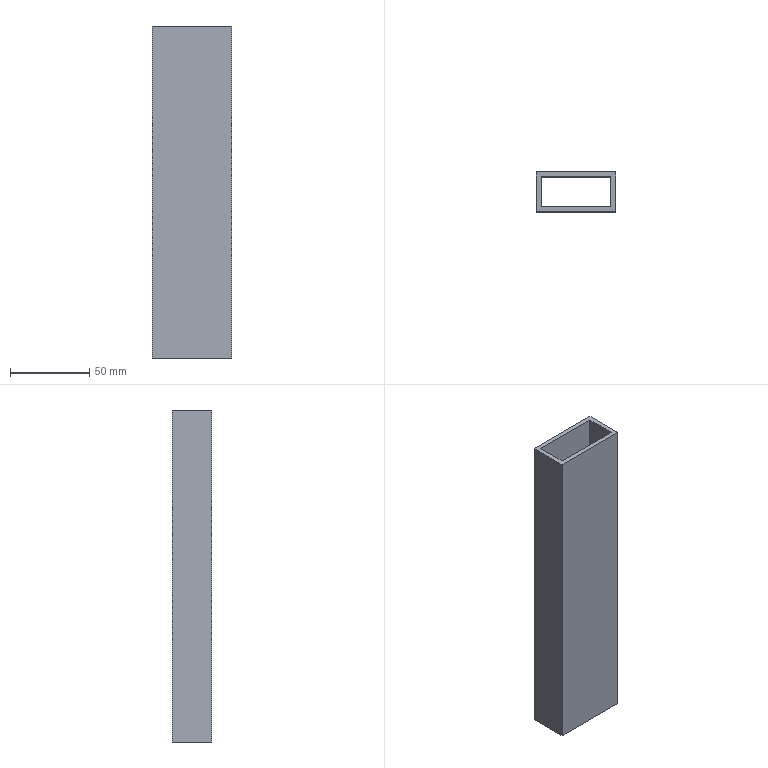Part | STEP file | ASND-0110-E63-HLTP01标准Lower机架-11 | 1 solid | 10 faces | box 50 x 25 x 210 mm | volume 86940 mm3 | plane 10
STEP:
#1=CARTESIAN_POINT('',(0.,0.,0.));
#2=DIRECTION('',(0.,0.,1.));
#3=DIRECTION('',(1.,0.,0.));
#4=AXIS2_PLACEMENT_3D('',#1,#2,#3);
#5=CARTESIAN_POINT('',(-145.,12.5,-210.));
#6=VERTEX_POINT('',#5);
#7=CARTESIAN_POINT('',(-95.,12.5,-210.));
#8=VERTEX_POINT('',#7);
#9=CARTESIAN_POINT('',(-145.,12.5,-210.));
#10=DIRECTION('',(1.,0.,0.));
#11=VECTOR('',#10,1.);
#12=LINE('',#9,#11);
#13=CARTESIAN_POINT('',(-95.,12.5,-265.902));
#14=DIRECTION('',(0.,1.,0.));
#15=DIRECTION('',(0.7071,0.,0.7071));
#16=AXIS2_PLACEMENT_3D('',#13,#14,#15);
#17=PLANE('',#16);
#18=CARTESIAN_POINT('',(4.173,-74.884));
#19=DIRECTION('',(0.7071,0.7071));
#20=VECTOR('',#19,1.);
#21=LINE('',#18,#20);
#22=(GEOMETRIC_REPRESENTATION_CONTEXT(2)PARAMETRIC_REPRESENTATION_CONTEXT()REPRESENTATION_CONTEXT('',''));
#23=DEFINITIONAL_REPRESENTATION('',(#21),#22);
#24=PCURVE('',#17,#23);
#25=CARTESIAN_POINT('',(-200.902,-12.5,-210.));
#26=DIRECTION('',(0.,0.,1.));
#27=DIRECTION('',(0.7071,0.7071,0.));
#28=AXIS2_PLACEMENT_3D('',#25,#26,#27);
#29=PLANE('',#28);
#30=CARTESIAN_POINT('',(57.206,-21.851));
#31=DIRECTION('',(0.7071,-0.7071));
#32=VECTOR('',#31,1.);
#33=LINE('',#30,#32);
#34=(GEOMETRIC_REPRESENTATION_CONTEXT(2)PARAMETRIC_REPRESENTATION_CONTEXT()REPRESENTATION_CONTEXT('',''));
#35=DEFINITIONAL_REPRESENTATION('',(#33),#34);
#36=PCURVE('',#29,#35);
#37=SURFACE_CURVE('',#12,(#24,#36),.PCURVE_S1.);
#38=EDGE_CURVE('',#6,#8,#37,.T.);
#39=ORIENTED_EDGE('',*,*,#38,.F.);
#40=CARTESIAN_POINT('',(-145.,12.5,0.));
#41=VERTEX_POINT('',#40);
#42=CARTESIAN_POINT('',(-145.,12.5,-210.));
#43=DIRECTION('',(0.,0.,1.));
#44=VECTOR('',#43,1.);
#45=LINE('',#42,#44);
#46=CARTESIAN_POINT('',(4.173,-74.884));
#47=DIRECTION('',(0.7071,-0.7071));
#48=VECTOR('',#47,1.);
#49=LINE('',#46,#48);
#50=(GEOMETRIC_REPRESENTATION_CONTEXT(2)PARAMETRIC_REPRESENTATION_CONTEXT()REPRESENTATION_CONTEXT('',''));
#51=DEFINITIONAL_REPRESENTATION('',(#49),#50);
#52=PCURVE('',#17,#51);
#53=CARTESIAN_POINT('',(-145.,12.5,-265.902));
#54=DIRECTION('',(-1.,0.,0.));
#55=DIRECTION('',(0.,0.7071,0.7071));
#56=AXIS2_PLACEMENT_3D('',#53,#54,#55);
#57=PLANE('',#56);
#58=CARTESIAN_POINT('',(39.528,-39.528));
#59=DIRECTION('',(0.7071,-0.7071));
#60=VECTOR('',#59,1.);
#61=LINE('',#58,#60);
#62=(GEOMETRIC_REPRESENTATION_CONTEXT(2)PARAMETRIC_REPRESENTATION_CONTEXT()REPRESENTATION_CONTEXT('',''));
#63=DEFINITIONAL_REPRESENTATION('',(#61),#62);
#64=PCURVE('',#57,#63);
#65=SURFACE_CURVE('',#45,(#52,#64),.PCURVE_S1.);
#66=EDGE_CURVE('',#6,#41,#65,.T.);
#67=ORIENTED_EDGE('',*,*,#66,.T.);
#68=CARTESIAN_POINT('',(-95.,12.5,0.));
#69=VERTEX_POINT('',#68);
#70=CARTESIAN_POINT('',(-95.,12.5,0.));
#71=DIRECTION('',(-1.,0.,0.));
#72=VECTOR('',#71,1.);
#73=LINE('',#70,#72);
#74=CARTESIAN_POINT('',(188.021,-188.021));
#75=DIRECTION('',(-0.7071,-0.7071));
#76=VECTOR('',#75,1.);
#77=LINE('',#74,#76);
#78=(GEOMETRIC_REPRESENTATION_CONTEXT(2)PARAMETRIC_REPRESENTATION_CONTEXT()REPRESENTATION_CONTEXT('',''));
#79=DEFINITIONAL_REPRESENTATION('',(#77),#78);
#80=PCURVE('',#17,#79);
#81=CARTESIAN_POINT('',(0.,0.,0.));
#82=DIRECTION('',(0.,0.,-1.));
#83=DIRECTION('',(0.7071,0.7071,0.));
#84=AXIS2_PLACEMENT_3D('',#81,#82,#83);
#85=PLANE('',#84);
#86=CARTESIAN_POINT('',(-58.336,-76.014));
#87=DIRECTION('',(-0.7071,-0.7071));
#88=VECTOR('',#87,1.);
#89=LINE('',#86,#88);
#90=(GEOMETRIC_REPRESENTATION_CONTEXT(2)PARAMETRIC_REPRESENTATION_CONTEXT()REPRESENTATION_CONTEXT('',''));
#91=DEFINITIONAL_REPRESENTATION('',(#89),#90);
#92=PCURVE('',#85,#91);
#93=SURFACE_CURVE('',#73,(#80,#92),.PCURVE_S1.);
#94=EDGE_CURVE('',#69,#41,#93,.T.);
#95=ORIENTED_EDGE('',*,*,#94,.F.);
#96=CARTESIAN_POINT('',(-95.,12.5,-210.));
#97=DIRECTION('',(0.,0.,1.));
#98=VECTOR('',#97,1.);
#99=LINE('',#96,#98);
#100=CARTESIAN_POINT('',(39.528,-39.528));
#101=DIRECTION('',(0.7071,-0.7071));
#102=VECTOR('',#101,1.);
#103=LINE('',#100,#102);
#104=(GEOMETRIC_REPRESENTATION_CONTEXT(2)PARAMETRIC_REPRESENTATION_CONTEXT()REPRESENTATION_CONTEXT('',''));
#105=DEFINITIONAL_REPRESENTATION('',(#103),#104);
#106=PCURVE('',#17,#105);
#107=CARTESIAN_POINT('',(-95.,12.5,-265.902));
#108=DIRECTION('',(1.,0.,0.));
#109=DIRECTION('',(0.,0.7071,0.7071));
#110=AXIS2_PLACEMENT_3D('',#107,#108,#109);
#111=PLANE('',#110);
#112=CARTESIAN_POINT('',(39.528,39.528));
#113=DIRECTION('',(0.7071,0.7071));
#114=VECTOR('',#113,1.);
#115=LINE('',#112,#114);
#116=(GEOMETRIC_REPRESENTATION_CONTEXT(2)PARAMETRIC_REPRESENTATION_CONTEXT()REPRESENTATION_CONTEXT('',''));
#117=DEFINITIONAL_REPRESENTATION('',(#115),#116);
#118=PCURVE('',#111,#117);
#119=SURFACE_CURVE('',#99,(#106,#118),.PCURVE_S1.);
#120=EDGE_CURVE('',#8,#69,#119,.T.);
#121=ORIENTED_EDGE('',*,*,#120,.F.);
#122=EDGE_LOOP('',(#39,#67,#95,#121));
#123=FACE_BOUND('',#122,.T.);
#124=ADVANCED_FACE('',(#123),#17,.T.);
#125=CARTESIAN_POINT('',(-145.,-12.5,-210.));
#126=VERTEX_POINT('',#125);
#127=CARTESIAN_POINT('',(-145.,-12.5,-210.));
#128=DIRECTION('',(0.,1.,0.));
#129=VECTOR('',#128,1.);
#130=LINE('',#127,#129);
#131=CARTESIAN_POINT('',(21.851,-57.206));
#132=DIRECTION('',(0.7071,0.7071));
#133=VECTOR('',#132,1.);
#134=LINE('',#131,#133);
#135=(GEOMETRIC_REPRESENTATION_CONTEXT(2)PARAMETRIC_REPRESENTATION_CONTEXT()REPRESENTATION_CONTEXT('',''));
#136=DEFINITIONAL_REPRESENTATION('',(#134),#135);
#137=PCURVE('',#57,#136);
#138=CARTESIAN_POINT('',(39.528,-39.528));
#139=DIRECTION('',(0.7071,0.7071));
#140=VECTOR('',#139,1.);
#141=LINE('',#138,#140);
#142=(GEOMETRIC_REPRESENTATION_CONTEXT(2)PARAMETRIC_REPRESENTATION_CONTEXT()REPRESENTATION_CONTEXT('',''));
#143=DEFINITIONAL_REPRESENTATION('',(#141),#142);
#144=PCURVE('',#29,#143);
#145=SURFACE_CURVE('',#130,(#137,#144),.PCURVE_S1.);
#146=EDGE_CURVE('',#126,#6,#145,.T.);
#147=ORIENTED_EDGE('',*,*,#146,.F.);
#148=CARTESIAN_POINT('',(-145.,-12.5,0.));
#149=VERTEX_POINT('',#148);
#150=CARTESIAN_POINT('',(-145.,-12.5,-210.));
#151=DIRECTION('',(0.,0.,1.));
#152=VECTOR('',#151,1.);
#153=LINE('',#150,#152);
#154=CARTESIAN_POINT('',(21.851,-57.206));
#155=DIRECTION('',(0.7071,-0.7071));
#156=VECTOR('',#155,1.);
#157=LINE('',#154,#156);
#158=(GEOMETRIC_REPRESENTATION_CONTEXT(2)PARAMETRIC_REPRESENTATION_CONTEXT()REPRESENTATION_CONTEXT('',''));
#159=DEFINITIONAL_REPRESENTATION('',(#157),#158);
#160=PCURVE('',#57,#159);
#161=CARTESIAN_POINT('',(-95.,-12.5,-265.902));
#162=DIRECTION('',(0.,-1.,0.));
#163=DIRECTION('',(0.7071,0.,0.7071));
#164=AXIS2_PLACEMENT_3D('',#161,#162,#163);
#165=PLANE('',#164);
#166=CARTESIAN_POINT('',(4.173,74.884));
#167=DIRECTION('',(0.7071,0.7071));
#168=VECTOR('',#167,1.);
#169=LINE('',#166,#168);
#170=(GEOMETRIC_REPRESENTATION_CONTEXT(2)PARAMETRIC_REPRESENTATION_CONTEXT()REPRESENTATION_CONTEXT('',''));
#171=DEFINITIONAL_REPRESENTATION('',(#169),#170);
#172=PCURVE('',#165,#171);
#173=SURFACE_CURVE('',#153,(#160,#172),.PCURVE_S1.);
#174=EDGE_CURVE('',#126,#149,#173,.T.);
#175=ORIENTED_EDGE('',*,*,#174,.T.);
#176=CARTESIAN_POINT('',(-145.,12.5,0.));
#177=DIRECTION('',(0.,-1.,0.));
#178=VECTOR('',#177,1.);
#179=LINE('',#176,#178);
#180=CARTESIAN_POINT('',(188.021,-188.021));
#181=DIRECTION('',(-0.7071,-0.7071));
#182=VECTOR('',#181,1.);
#183=LINE('',#180,#182);
#184=(GEOMETRIC_REPRESENTATION_CONTEXT(2)PARAMETRIC_REPRESENTATION_CONTEXT()REPRESENTATION_CONTEXT('',''));
#185=DEFINITIONAL_REPRESENTATION('',(#183),#184);
#186=PCURVE('',#57,#185);
#187=CARTESIAN_POINT('',(-93.692,-111.369));
#188=DIRECTION('',(-0.7071,0.7071));
#189=VECTOR('',#188,1.);
#190=LINE('',#187,#189);
#191=(GEOMETRIC_REPRESENTATION_CONTEXT(2)PARAMETRIC_REPRESENTATION_CONTEXT()REPRESENTATION_CONTEXT('',''));
#192=DEFINITIONAL_REPRESENTATION('',(#190),#191);
#193=PCURVE('',#85,#192);
#194=SURFACE_CURVE('',#179,(#186,#193),.PCURVE_S1.);
#195=EDGE_CURVE('',#41,#149,#194,.T.);
#196=ORIENTED_EDGE('',*,*,#195,.F.);
#197=ORIENTED_EDGE('',*,*,#66,.F.);
#198=EDGE_LOOP('',(#147,#175,#196,#197));
#199=FACE_BOUND('',#198,.T.);
#200=ADVANCED_FACE('',(#199),#57,.T.);
#201=CARTESIAN_POINT('',(-95.,-12.5,-210.));
#202=VERTEX_POINT('',#201);
#203=CARTESIAN_POINT('',(-95.,-12.5,-210.));
#204=DIRECTION('',(-1.,0.,0.));
#205=VECTOR('',#204,1.);
#206=LINE('',#203,#205);
#207=CARTESIAN_POINT('',(39.528,39.528));
#208=DIRECTION('',(-0.7071,0.7071));
#209=VECTOR('',#208,1.);
#210=LINE('',#207,#209);
#211=(GEOMETRIC_REPRESENTATION_CONTEXT(2)PARAMETRIC_REPRESENTATION_CONTEXT()REPRESENTATION_CONTEXT('',''));
#212=DEFINITIONAL_REPRESENTATION('',(#210),#211);
#213=PCURVE('',#165,#212);
#214=CARTESIAN_POINT('',(74.884,-74.884));
#215=DIRECTION('',(-0.7071,0.7071));
#216=VECTOR('',#215,1.);
#217=LINE('',#214,#216);
#218=(GEOMETRIC_REPRESENTATION_CONTEXT(2)PARAMETRIC_REPRESENTATION_CONTEXT()REPRESENTATION_CONTEXT('',''));
#219=DEFINITIONAL_REPRESENTATION('',(#217),#218);
#220=PCURVE('',#29,#219);
#221=SURFACE_CURVE('',#206,(#213,#220),.PCURVE_S1.);
#222=EDGE_CURVE('',#202,#126,#221,.T.);
#223=ORIENTED_EDGE('',*,*,#222,.F.);
#224=CARTESIAN_POINT('',(-95.,-12.5,0.));
#225=VERTEX_POINT('',#224);
#226=CARTESIAN_POINT('',(-95.,-12.5,-210.));
#227=DIRECTION('',(0.,0.,1.));
#228=VECTOR('',#227,1.);
#229=LINE('',#226,#228);
#230=CARTESIAN_POINT('',(39.528,39.528));
#231=DIRECTION('',(0.7071,0.7071));
#232=VECTOR('',#231,1.);
#233=LINE('',#230,#232);
#234=(GEOMETRIC_REPRESENTATION_CONTEXT(2)PARAMETRIC_REPRESENTATION_CONTEXT()REPRESENTATION_CONTEXT('',''));
#235=DEFINITIONAL_REPRESENTATION('',(#233),#234);
#236=PCURVE('',#165,#235);
#237=CARTESIAN_POINT('',(21.851,57.206));
#238=DIRECTION('',(0.7071,0.7071));
#239=VECTOR('',#238,1.);
#240=LINE('',#237,#239);
#241=(GEOMETRIC_REPRESENTATION_CONTEXT(2)PARAMETRIC_REPRESENTATION_CONTEXT()REPRESENTATION_CONTEXT('',''));
#242=DEFINITIONAL_REPRESENTATION('',(#240),#241);
#243=PCURVE('',#111,#242);
#244=SURFACE_CURVE('',#229,(#236,#243),.PCURVE_S1.);
#245=EDGE_CURVE('',#202,#225,#244,.T.);
#246=ORIENTED_EDGE('',*,*,#245,.T.);
#247=CARTESIAN_POINT('',(-145.,-12.5,0.));
#248=DIRECTION('',(1.,0.,0.));
#249=VECTOR('',#248,1.);
#250=LINE('',#247,#249);
#251=CARTESIAN_POINT('',(152.666,223.376));
#252=DIRECTION('',(0.7071,-0.7071));
#253=VECTOR('',#252,1.);
#254=LINE('',#251,#253);
#255=(GEOMETRIC_REPRESENTATION_CONTEXT(2)PARAMETRIC_REPRESENTATION_CONTEXT()REPRESENTATION_CONTEXT('',''));
#256=DEFINITIONAL_REPRESENTATION('',(#254),#255);
#257=PCURVE('',#165,#256);
#258=CARTESIAN_POINT('',(-111.369,-93.692));
#259=DIRECTION('',(0.7071,0.7071));
#260=VECTOR('',#259,1.);
#261=LINE('',#258,#260);
#262=(GEOMETRIC_REPRESENTATION_CONTEXT(2)PARAMETRIC_REPRESENTATION_CONTEXT()REPRESENTATION_CONTEXT('',''));
#263=DEFINITIONAL_REPRESENTATION('',(#261),#262);
#264=PCURVE('',#85,#263);
#265=SURFACE_CURVE('',#250,(#257,#264),.PCURVE_S1.);
#266=EDGE_CURVE('',#149,#225,#265,.T.);
#267=ORIENTED_EDGE('',*,*,#266,.F.);
#268=ORIENTED_EDGE('',*,*,#174,.F.);
#269=EDGE_LOOP('',(#223,#246,#267,#268));
#270=FACE_BOUND('',#269,.T.);
#271=ADVANCED_FACE('',(#270),#165,.T.);
#272=CARTESIAN_POINT('',(-95.,12.5,-210.));
#273=DIRECTION('',(0.,-1.,0.));
#274=VECTOR('',#273,1.);
#275=LINE('',#272,#274);
#276=CARTESIAN_POINT('',(39.528,39.528));
#277=DIRECTION('',(-0.7071,0.7071));
#278=VECTOR('',#277,1.);
#279=LINE('',#276,#278);
#280=(GEOMETRIC_REPRESENTATION_CONTEXT(2)PARAMETRIC_REPRESENTATION_CONTEXT()REPRESENTATION_CONTEXT('',''));
#281=DEFINITIONAL_REPRESENTATION('',(#279),#280);
#282=PCURVE('',#111,#281);
#283=CARTESIAN_POINT('',(92.561,-57.206));
#284=DIRECTION('',(-0.7071,-0.7071));
#285=VECTOR('',#284,1.);
#286=LINE('',#283,#285);
#287=(GEOMETRIC_REPRESENTATION_CONTEXT(2)PARAMETRIC_REPRESENTATION_CONTEXT()REPRESENTATION_CONTEXT('',''));
#288=DEFINITIONAL_REPRESENTATION('',(#286),#287);
#289=PCURVE('',#29,#288);
#290=SURFACE_CURVE('',#275,(#282,#289),.PCURVE_S1.);
#291=EDGE_CURVE('',#8,#202,#290,.T.);
#292=ORIENTED_EDGE('',*,*,#291,.F.);
#293=ORIENTED_EDGE('',*,*,#120,.T.);
#294=CARTESIAN_POINT('',(-95.,-12.5,0.));
#295=DIRECTION('',(0.,1.,0.));
#296=VECTOR('',#295,1.);
#297=LINE('',#294,#296);
#298=CARTESIAN_POINT('',(170.343,205.699));
#299=DIRECTION('',(0.7071,-0.7071));
#300=VECTOR('',#299,1.);
#301=LINE('',#298,#300);
#302=(GEOMETRIC_REPRESENTATION_CONTEXT(2)PARAMETRIC_REPRESENTATION_CONTEXT()REPRESENTATION_CONTEXT('',''));
#303=DEFINITIONAL_REPRESENTATION('',(#301),#302);
#304=PCURVE('',#111,#303);
#305=CARTESIAN_POINT('',(-76.014,-58.336));
#306=DIRECTION('',(0.7071,-0.7071));
#307=VECTOR('',#306,1.);
#308=LINE('',#305,#307);
#309=(GEOMETRIC_REPRESENTATION_CONTEXT(2)PARAMETRIC_REPRESENTATION_CONTEXT()REPRESENTATION_CONTEXT('',''));
#310=DEFINITIONAL_REPRESENTATION('',(#308),#309);
#311=PCURVE('',#85,#310);
#312=SURFACE_CURVE('',#297,(#304,#311),.PCURVE_S1.);
#313=EDGE_CURVE('',#225,#69,#312,.T.);
#314=ORIENTED_EDGE('',*,*,#313,.F.);
#315=ORIENTED_EDGE('',*,*,#245,.F.);
#316=EDGE_LOOP('',(#292,#293,#314,#315));
#317=FACE_BOUND('',#316,.T.);
#318=ADVANCED_FACE('',(#317),#111,.T.);
#319=ORIENTED_EDGE('',*,*,#313,.T.);
#320=ORIENTED_EDGE('',*,*,#94,.T.);
#321=ORIENTED_EDGE('',*,*,#195,.T.);
#322=ORIENTED_EDGE('',*,*,#266,.T.);
#323=EDGE_LOOP('',(#319,#320,#321,#322));
#324=FACE_BOUND('',#323,.T.);
#325=CARTESIAN_POINT('',(-98.,9.5,0.));
#326=VERTEX_POINT('',#325);
#327=CARTESIAN_POINT('',(-142.,9.5,0.));
#328=VERTEX_POINT('',#327);
#329=CARTESIAN_POINT('',(-98.,9.5,0.));
#330=DIRECTION('',(-1.,0.,0.));
#331=VECTOR('',#330,1.);
#332=LINE('',#329,#331);
#333=CARTESIAN_POINT('',(-62.579,-76.014));
#334=DIRECTION('',(-0.7071,-0.7071));
#335=VECTOR('',#334,1.);
#336=LINE('',#333,#335);
#337=(GEOMETRIC_REPRESENTATION_CONTEXT(2)PARAMETRIC_REPRESENTATION_CONTEXT()REPRESENTATION_CONTEXT('',''));
#338=DEFINITIONAL_REPRESENTATION('',(#336),#337);
#339=PCURVE('',#85,#338);
#340=CARTESIAN_POINT('',(-98.,9.5,-265.902));
#341=DIRECTION('',(0.,1.,0.));
#342=DIRECTION('',(0.7071,0.,0.7071));
#343=AXIS2_PLACEMENT_3D('',#340,#341,#342);
#344=PLANE('',#343);
#345=CARTESIAN_POINT('',(188.021,-188.021));
#346=DIRECTION('',(-0.7071,-0.7071));
#347=VECTOR('',#346,1.);
#348=LINE('',#345,#347);
#349=(GEOMETRIC_REPRESENTATION_CONTEXT(2)PARAMETRIC_REPRESENTATION_CONTEXT()REPRESENTATION_CONTEXT('',''));
#350=DEFINITIONAL_REPRESENTATION('',(#348),#349);
#351=PCURVE('',#344,#350);
#352=SURFACE_CURVE('',#332,(#339,#351),.PCURVE_S1.);
#353=EDGE_CURVE('',#326,#328,#352,.T.);
#354=ORIENTED_EDGE('',*,*,#353,.F.);
#355=CARTESIAN_POINT('',(-98.,-9.5,0.));
#356=VERTEX_POINT('',#355);
#357=CARTESIAN_POINT('',(-98.,-9.5,0.));
#358=DIRECTION('',(0.,1.,0.));
#359=VECTOR('',#358,1.);
#360=LINE('',#357,#359);
#361=CARTESIAN_POINT('',(-76.014,-62.579));
#362=DIRECTION('',(0.7071,-0.7071));
#363=VECTOR('',#362,1.);
#364=LINE('',#361,#363);
#365=(GEOMETRIC_REPRESENTATION_CONTEXT(2)PARAMETRIC_REPRESENTATION_CONTEXT()REPRESENTATION_CONTEXT('',''));
#366=DEFINITIONAL_REPRESENTATION('',(#364),#365);
#367=PCURVE('',#85,#366);
#368=CARTESIAN_POINT('',(-98.,9.5,-265.902));
#369=DIRECTION('',(1.,0.,0.));
#370=DIRECTION('',(0.,0.7071,0.7071));
#371=AXIS2_PLACEMENT_3D('',#368,#369,#370);
#372=PLANE('',#371);
#373=CARTESIAN_POINT('',(174.586,201.456));
#374=DIRECTION('',(0.7071,-0.7071));
#375=VECTOR('',#374,1.);
#376=LINE('',#373,#375);
#377=(GEOMETRIC_REPRESENTATION_CONTEXT(2)PARAMETRIC_REPRESENTATION_CONTEXT()REPRESENTATION_CONTEXT('',''));
#378=DEFINITIONAL_REPRESENTATION('',(#376),#377);
#379=PCURVE('',#372,#378);
#380=SURFACE_CURVE('',#360,(#367,#379),.PCURVE_S1.);
#381=EDGE_CURVE('',#356,#326,#380,.T.);
#382=ORIENTED_EDGE('',*,*,#381,.F.);
#383=CARTESIAN_POINT('',(-142.,-9.5,0.));
#384=VERTEX_POINT('',#383);
#385=CARTESIAN_POINT('',(-142.,-9.5,0.));
#386=DIRECTION('',(1.,0.,0.));
#387=VECTOR('',#386,1.);
#388=LINE('',#385,#387);
#389=CARTESIAN_POINT('',(-107.127,-93.692));
#390=DIRECTION('',(0.7071,0.7071));
#391=VECTOR('',#390,1.);
#392=LINE('',#389,#391);
#393=(GEOMETRIC_REPRESENTATION_CONTEXT(2)PARAMETRIC_REPRESENTATION_CONTEXT()REPRESENTATION_CONTEXT('',''));
#394=DEFINITIONAL_REPRESENTATION('',(#392),#393);
#395=PCURVE('',#85,#394);
#396=CARTESIAN_POINT('',(-98.,-9.5,-265.902));
#397=DIRECTION('',(0.,-1.,0.));
#398=DIRECTION('',(0.7071,0.,0.7071));
#399=AXIS2_PLACEMENT_3D('',#396,#397,#398);
#400=PLANE('',#399);
#401=CARTESIAN_POINT('',(156.908,219.134));
#402=DIRECTION('',(0.7071,-0.7071));
#403=VECTOR('',#402,1.);
#404=LINE('',#401,#403);
#405=(GEOMETRIC_REPRESENTATION_CONTEXT(2)PARAMETRIC_REPRESENTATION_CONTEXT()REPRESENTATION_CONTEXT('',''));
#406=DEFINITIONAL_REPRESENTATION('',(#404),#405);
#407=PCURVE('',#400,#406);
#408=SURFACE_CURVE('',#388,(#395,#407),.PCURVE_S1.);
#409=EDGE_CURVE('',#384,#356,#408,.T.);
#410=ORIENTED_EDGE('',*,*,#409,.F.);
#411=CARTESIAN_POINT('',(-142.,9.5,0.));
#412=DIRECTION('',(0.,-1.,0.));
#413=VECTOR('',#412,1.);
#414=LINE('',#411,#413);
#415=CARTESIAN_POINT('',(-93.692,-107.127));
#416=DIRECTION('',(-0.7071,0.7071));
#417=VECTOR('',#416,1.);
#418=LINE('',#415,#417);
#419=(GEOMETRIC_REPRESENTATION_CONTEXT(2)PARAMETRIC_REPRESENTATION_CONTEXT()REPRESENTATION_CONTEXT('',''));
#420=DEFINITIONAL_REPRESENTATION('',(#418),#419);
#421=PCURVE('',#85,#420);
#422=CARTESIAN_POINT('',(-142.,9.5,-265.902));
#423=DIRECTION('',(-1.,0.,0.));
#424=DIRECTION('',(0.,0.7071,0.7071));
#425=AXIS2_PLACEMENT_3D('',#422,#423,#424);
#426=PLANE('',#425);
#427=CARTESIAN_POINT('',(188.021,-188.021));
#428=DIRECTION('',(-0.7071,-0.7071));
#429=VECTOR('',#428,1.);
#430=LINE('',#427,#429);
#431=(GEOMETRIC_REPRESENTATION_CONTEXT(2)PARAMETRIC_REPRESENTATION_CONTEXT()REPRESENTATION_CONTEXT('',''));
#432=DEFINITIONAL_REPRESENTATION('',(#430),#431);
#433=PCURVE('',#426,#432);
#434=SURFACE_CURVE('',#414,(#421,#433),.PCURVE_S1.);
#435=EDGE_CURVE('',#328,#384,#434,.T.);
#436=ORIENTED_EDGE('',*,*,#435,.F.);
#437=EDGE_LOOP('',(#354,#382,#410,#436));
#438=FACE_BOUND('',#437,.T.);
#439=ADVANCED_FACE('',(#324,#438),#85,.F.);
#440=CARTESIAN_POINT('',(-142.,9.5,-210.));
#441=VERTEX_POINT('',#440);
#442=CARTESIAN_POINT('',(-142.,9.5,-210.));
#443=DIRECTION('',(0.,0.,1.));
#444=VECTOR('',#443,1.);
#445=LINE('',#442,#444);
#446=CARTESIAN_POINT('',(8.416,-70.641));
#447=DIRECTION('',(0.7071,-0.7071));
#448=VECTOR('',#447,1.);
#449=LINE('',#446,#448);
#450=(GEOMETRIC_REPRESENTATION_CONTEXT(2)PARAMETRIC_REPRESENTATION_CONTEXT()REPRESENTATION_CONTEXT('',''));
#451=DEFINITIONAL_REPRESENTATION('',(#449),#450);
#452=PCURVE('',#344,#451);
#453=CARTESIAN_POINT('',(39.528,-39.528));
#454=DIRECTION('',(0.7071,-0.7071));
#455=VECTOR('',#454,1.);
#456=LINE('',#453,#455);
#457=(GEOMETRIC_REPRESENTATION_CONTEXT(2)PARAMETRIC_REPRESENTATION_CONTEXT()REPRESENTATION_CONTEXT('',''));
#458=DEFINITIONAL_REPRESENTATION('',(#456),#457);
#459=PCURVE('',#426,#458);
#460=SURFACE_CURVE('',#445,(#452,#459),.PCURVE_S1.);
#461=EDGE_CURVE('',#441,#328,#460,.T.);
#462=ORIENTED_EDGE('',*,*,#461,.F.);
#463=CARTESIAN_POINT('',(-98.,9.5,-210.));
#464=VERTEX_POINT('',#463);
#465=CARTESIAN_POINT('',(-142.,9.5,-210.));
#466=DIRECTION('',(1.,0.,0.));
#467=VECTOR('',#466,1.);
#468=LINE('',#465,#467);
#469=CARTESIAN_POINT('',(8.416,-70.641));
#470=DIRECTION('',(0.7071,0.7071));
#471=VECTOR('',#470,1.);
#472=LINE('',#469,#471);
#473=(GEOMETRIC_REPRESENTATION_CONTEXT(2)PARAMETRIC_REPRESENTATION_CONTEXT()REPRESENTATION_CONTEXT('',''));
#474=DEFINITIONAL_REPRESENTATION('',(#472),#473);
#475=PCURVE('',#344,#474);
#476=CARTESIAN_POINT('',(57.206,-26.093));
#477=DIRECTION('',(0.7071,-0.7071));
#478=VECTOR('',#477,1.);
#479=LINE('',#476,#478);
#480=(GEOMETRIC_REPRESENTATION_CONTEXT(2)PARAMETRIC_REPRESENTATION_CONTEXT()REPRESENTATION_CONTEXT('',''));
#481=DEFINITIONAL_REPRESENTATION('',(#479),#480);
#482=PCURVE('',#29,#481);
#483=SURFACE_CURVE('',#468,(#475,#482),.PCURVE_S1.);
#484=EDGE_CURVE('',#441,#464,#483,.T.);
#485=ORIENTED_EDGE('',*,*,#484,.T.);
#486=CARTESIAN_POINT('',(-98.,9.5,-210.));
#487=DIRECTION('',(0.,0.,1.));
#488=VECTOR('',#487,1.);
#489=LINE('',#486,#488);
#490=CARTESIAN_POINT('',(39.528,-39.528));
#491=DIRECTION('',(0.7071,-0.7071));
#492=VECTOR('',#491,1.);
#493=LINE('',#490,#492);
#494=(GEOMETRIC_REPRESENTATION_CONTEXT(2)PARAMETRIC_REPRESENTATION_CONTEXT()REPRESENTATION_CONTEXT('',''));
#495=DEFINITIONAL_REPRESENTATION('',(#493),#494);
#496=PCURVE('',#344,#495);
#497=CARTESIAN_POINT('',(39.528,39.528));
#498=DIRECTION('',(0.7071,0.7071));
#499=VECTOR('',#498,1.);
#500=LINE('',#497,#499);
#501=(GEOMETRIC_REPRESENTATION_CONTEXT(2)PARAMETRIC_REPRESENTATION_CONTEXT()REPRESENTATION_CONTEXT('',''));
#502=DEFINITIONAL_REPRESENTATION('',(#500),#501);
#503=PCURVE('',#372,#502);
#504=SURFACE_CURVE('',#489,(#496,#503),.PCURVE_S1.);
#505=EDGE_CURVE('',#464,#326,#504,.T.);
#506=ORIENTED_EDGE('',*,*,#505,.T.);
#507=ORIENTED_EDGE('',*,*,#353,.T.);
#508=EDGE_LOOP('',(#462,#485,#506,#507));
#509=FACE_BOUND('',#508,.T.);
#510=ADVANCED_FACE('',(#509),#344,.F.);
#511=CARTESIAN_POINT('',(-142.,-9.5,-210.));
#512=VERTEX_POINT('',#511);
#513=CARTESIAN_POINT('',(-142.,-9.5,-210.));
#514=DIRECTION('',(0.,0.,1.));
#515=VECTOR('',#514,1.);
#516=LINE('',#513,#515);
#517=CARTESIAN_POINT('',(26.093,-52.963));
#518=DIRECTION('',(0.7071,-0.7071));
#519=VECTOR('',#518,1.);
#520=LINE('',#517,#519);
#521=(GEOMETRIC_REPRESENTATION_CONTEXT(2)PARAMETRIC_REPRESENTATION_CONTEXT()REPRESENTATION_CONTEXT('',''));
#522=DEFINITIONAL_REPRESENTATION('',(#520),#521);
#523=PCURVE('',#426,#522);
#524=CARTESIAN_POINT('',(8.416,70.641));
#525=DIRECTION('',(0.7071,0.7071));
#526=VECTOR('',#525,1.);
#527=LINE('',#524,#526);
#528=(GEOMETRIC_REPRESENTATION_CONTEXT(2)PARAMETRIC_REPRESENTATION_CONTEXT()REPRESENTATION_CONTEXT('',''));
#529=DEFINITIONAL_REPRESENTATION('',(#527),#528);
#530=PCURVE('',#400,#529);
#531=SURFACE_CURVE('',#516,(#523,#530),.PCURVE_S1.);
#532=EDGE_CURVE('',#512,#384,#531,.T.);
#533=ORIENTED_EDGE('',*,*,#532,.F.);
#534=CARTESIAN_POINT('',(-142.,-9.5,-210.));
#535=DIRECTION('',(0.,1.,0.));
#536=VECTOR('',#535,1.);
#537=LINE('',#534,#536);
#538=CARTESIAN_POINT('',(26.093,-52.963));
#539=DIRECTION('',(0.7071,0.7071));
#540=VECTOR('',#539,1.);
#541=LINE('',#538,#540);
#542=(GEOMETRIC_REPRESENTATION_CONTEXT(2)PARAMETRIC_REPRESENTATION_CONTEXT()REPRESENTATION_CONTEXT('',''));
#543=DEFINITIONAL_REPRESENTATION('',(#541),#542);
#544=PCURVE('',#426,#543);
#545=CARTESIAN_POINT('',(43.771,-39.528));
#546=DIRECTION('',(0.7071,0.7071));
#547=VECTOR('',#546,1.);
#548=LINE('',#545,#547);
#549=(GEOMETRIC_REPRESENTATION_CONTEXT(2)PARAMETRIC_REPRESENTATION_CONTEXT()REPRESENTATION_CONTEXT('',''));
#550=DEFINITIONAL_REPRESENTATION('',(#548),#549);
#551=PCURVE('',#29,#550);
#552=SURFACE_CURVE('',#537,(#544,#551),.PCURVE_S1.);
#553=EDGE_CURVE('',#512,#441,#552,.T.);
#554=ORIENTED_EDGE('',*,*,#553,.T.);
#555=ORIENTED_EDGE('',*,*,#461,.T.);
#556=ORIENTED_EDGE('',*,*,#435,.T.);
#557=EDGE_LOOP('',(#533,#554,#555,#556));
#558=FACE_BOUND('',#557,.T.);
#559=ADVANCED_FACE('',(#558),#426,.F.);
#560=CARTESIAN_POINT('',(-98.,-9.5,-210.));
#561=VERTEX_POINT('',#560);
#562=CARTESIAN_POINT('',(-98.,-9.5,-210.));
#563=DIRECTION('',(0.,0.,1.));
#564=VECTOR('',#563,1.);
#565=LINE('',#562,#564);
#566=CARTESIAN_POINT('',(39.528,39.528));
#567=DIRECTION('',(0.7071,0.7071));
#568=VECTOR('',#567,1.);
#569=LINE('',#566,#568);
#570=(GEOMETRIC_REPRESENTATION_CONTEXT(2)PARAMETRIC_REPRESENTATION_CONTEXT()REPRESENTATION_CONTEXT('',''));
#571=DEFINITIONAL_REPRESENTATION('',(#569),#570);
#572=PCURVE('',#400,#571);
#573=CARTESIAN_POINT('',(26.093,52.963));
#574=DIRECTION('',(0.7071,0.7071));
#575=VECTOR('',#574,1.);
#576=LINE('',#573,#575);
#577=(GEOMETRIC_REPRESENTATION_CONTEXT(2)PARAMETRIC_REPRESENTATION_CONTEXT()REPRESENTATION_CONTEXT('',''));
#578=DEFINITIONAL_REPRESENTATION('',(#576),#577);
#579=PCURVE('',#372,#578);
#580=SURFACE_CURVE('',#565,(#572,#579),.PCURVE_S1.);
#581=EDGE_CURVE('',#561,#356,#580,.T.);
#582=ORIENTED_EDGE('',*,*,#581,.F.);
#583=CARTESIAN_POINT('',(-98.,-9.5,-210.));
#584=DIRECTION('',(-1.,0.,0.));
#585=VECTOR('',#584,1.);
#586=LINE('',#583,#585);
#587=CARTESIAN_POINT('',(39.528,39.528));
#588=DIRECTION('',(-0.7071,0.7071));
#589=VECTOR('',#588,1.);
#590=LINE('',#587,#589);
#591=(GEOMETRIC_REPRESENTATION_CONTEXT(2)PARAMETRIC_REPRESENTATION_CONTEXT()REPRESENTATION_CONTEXT('',''));
#592=DEFINITIONAL_REPRESENTATION('',(#590),#591);
#593=PCURVE('',#400,#592);
#594=CARTESIAN_POINT('',(74.884,-70.641));
#595=DIRECTION('',(-0.7071,0.7071));
#596=VECTOR('',#595,1.);
#597=LINE('',#594,#596);
#598=(GEOMETRIC_REPRESENTATION_CONTEXT(2)PARAMETRIC_REPRESENTATION_CONTEXT()REPRESENTATION_CONTEXT('',''));
#599=DEFINITIONAL_REPRESENTATION('',(#597),#598);
#600=PCURVE('',#29,#599);
#601=SURFACE_CURVE('',#586,(#593,#600),.PCURVE_S1.);
#602=EDGE_CURVE('',#561,#512,#601,.T.);
#603=ORIENTED_EDGE('',*,*,#602,.T.);
#604=ORIENTED_EDGE('',*,*,#532,.T.);
#605=ORIENTED_EDGE('',*,*,#409,.T.);
#606=EDGE_LOOP('',(#582,#603,#604,#605));
#607=FACE_BOUND('',#606,.T.);
#608=ADVANCED_FACE('',(#607),#400,.F.);
#609=ORIENTED_EDGE('',*,*,#505,.F.);
#610=CARTESIAN_POINT('',(-98.,9.5,-210.));
#611=DIRECTION('',(0.,-1.,0.));
#612=VECTOR('',#611,1.);
#613=LINE('',#610,#612);
#614=CARTESIAN_POINT('',(39.528,39.528));
#615=DIRECTION('',(-0.7071,0.7071));
#616=VECTOR('',#615,1.);
#617=LINE('',#614,#616);
#618=(GEOMETRIC_REPRESENTATION_CONTEXT(2)PARAMETRIC_REPRESENTATION_CONTEXT()REPRESENTATION_CONTEXT('',''));
#619=DEFINITIONAL_REPRESENTATION('',(#617),#618);
#620=PCURVE('',#372,#619);
#621=CARTESIAN_POINT('',(88.319,-57.206));
#622=DIRECTION('',(-0.7071,-0.7071));
#623=VECTOR('',#622,1.);
#624=LINE('',#621,#623);
#625=(GEOMETRIC_REPRESENTATION_CONTEXT(2)PARAMETRIC_REPRESENTATION_CONTEXT()REPRESENTATION_CONTEXT('',''));
#626=DEFINITIONAL_REPRESENTATION('',(#624),#625);
#627=PCURVE('',#29,#626);
#628=SURFACE_CURVE('',#613,(#620,#627),.PCURVE_S1.);
#629=EDGE_CURVE('',#464,#561,#628,.T.);
#630=ORIENTED_EDGE('',*,*,#629,.T.);
#631=ORIENTED_EDGE('',*,*,#581,.T.);
#632=ORIENTED_EDGE('',*,*,#381,.T.);
#633=EDGE_LOOP('',(#609,#630,#631,#632));
#634=FACE_BOUND('',#633,.T.);
#635=ADVANCED_FACE('',(#634),#372,.F.);
#636=ORIENTED_EDGE('',*,*,#291,.T.);
#637=ORIENTED_EDGE('',*,*,#222,.T.);
#638=ORIENTED_EDGE('',*,*,#146,.T.);
#639=ORIENTED_EDGE('',*,*,#38,.T.);
#640=EDGE_LOOP('',(#636,#637,#638,#639));
#641=FACE_BOUND('',#640,.T.);
#642=ORIENTED_EDGE('',*,*,#484,.F.);
#643=ORIENTED_EDGE('',*,*,#553,.F.);
#644=ORIENTED_EDGE('',*,*,#602,.F.);
#645=ORIENTED_EDGE('',*,*,#629,.F.);
#646=EDGE_LOOP('',(#642,#643,#644,#645));
#647=FACE_BOUND('',#646,.T.);
#648=ADVANCED_FACE('',(#641,#647),#29,.F.);
#649=CLOSED_SHELL('',(#124,#200,#271,#318,#439,#510,#559,#608,#635,#648));
#650=MANIFOLD_SOLID_BREP('',#649);
#651=(LENGTH_UNIT()NAMED_UNIT(*)SI_UNIT(.MILLI.,.METRE.));
#652=UNCERTAINTY_MEASURE_WITH_UNIT(LENGTH_MEASURE(0.0000001),#651,'','');
#653=(NAMED_UNIT(*)PLANE_ANGLE_UNIT()SI_UNIT($,.RADIAN.));
#654=(NAMED_UNIT(*)SI_UNIT($,.STERADIAN.)SOLID_ANGLE_UNIT());
#655=(GEOMETRIC_REPRESENTATION_CONTEXT(3)GLOBAL_UNCERTAINTY_ASSIGNED_CONTEXT((#652))GLOBAL_UNIT_ASSIGNED_CONTEXT((#651,#653,#654))REPRESENTATION_CONTEXT('',''));
#656=ADVANCED_BREP_SHAPE_REPRESENTATION('',(#4,#650),#655);